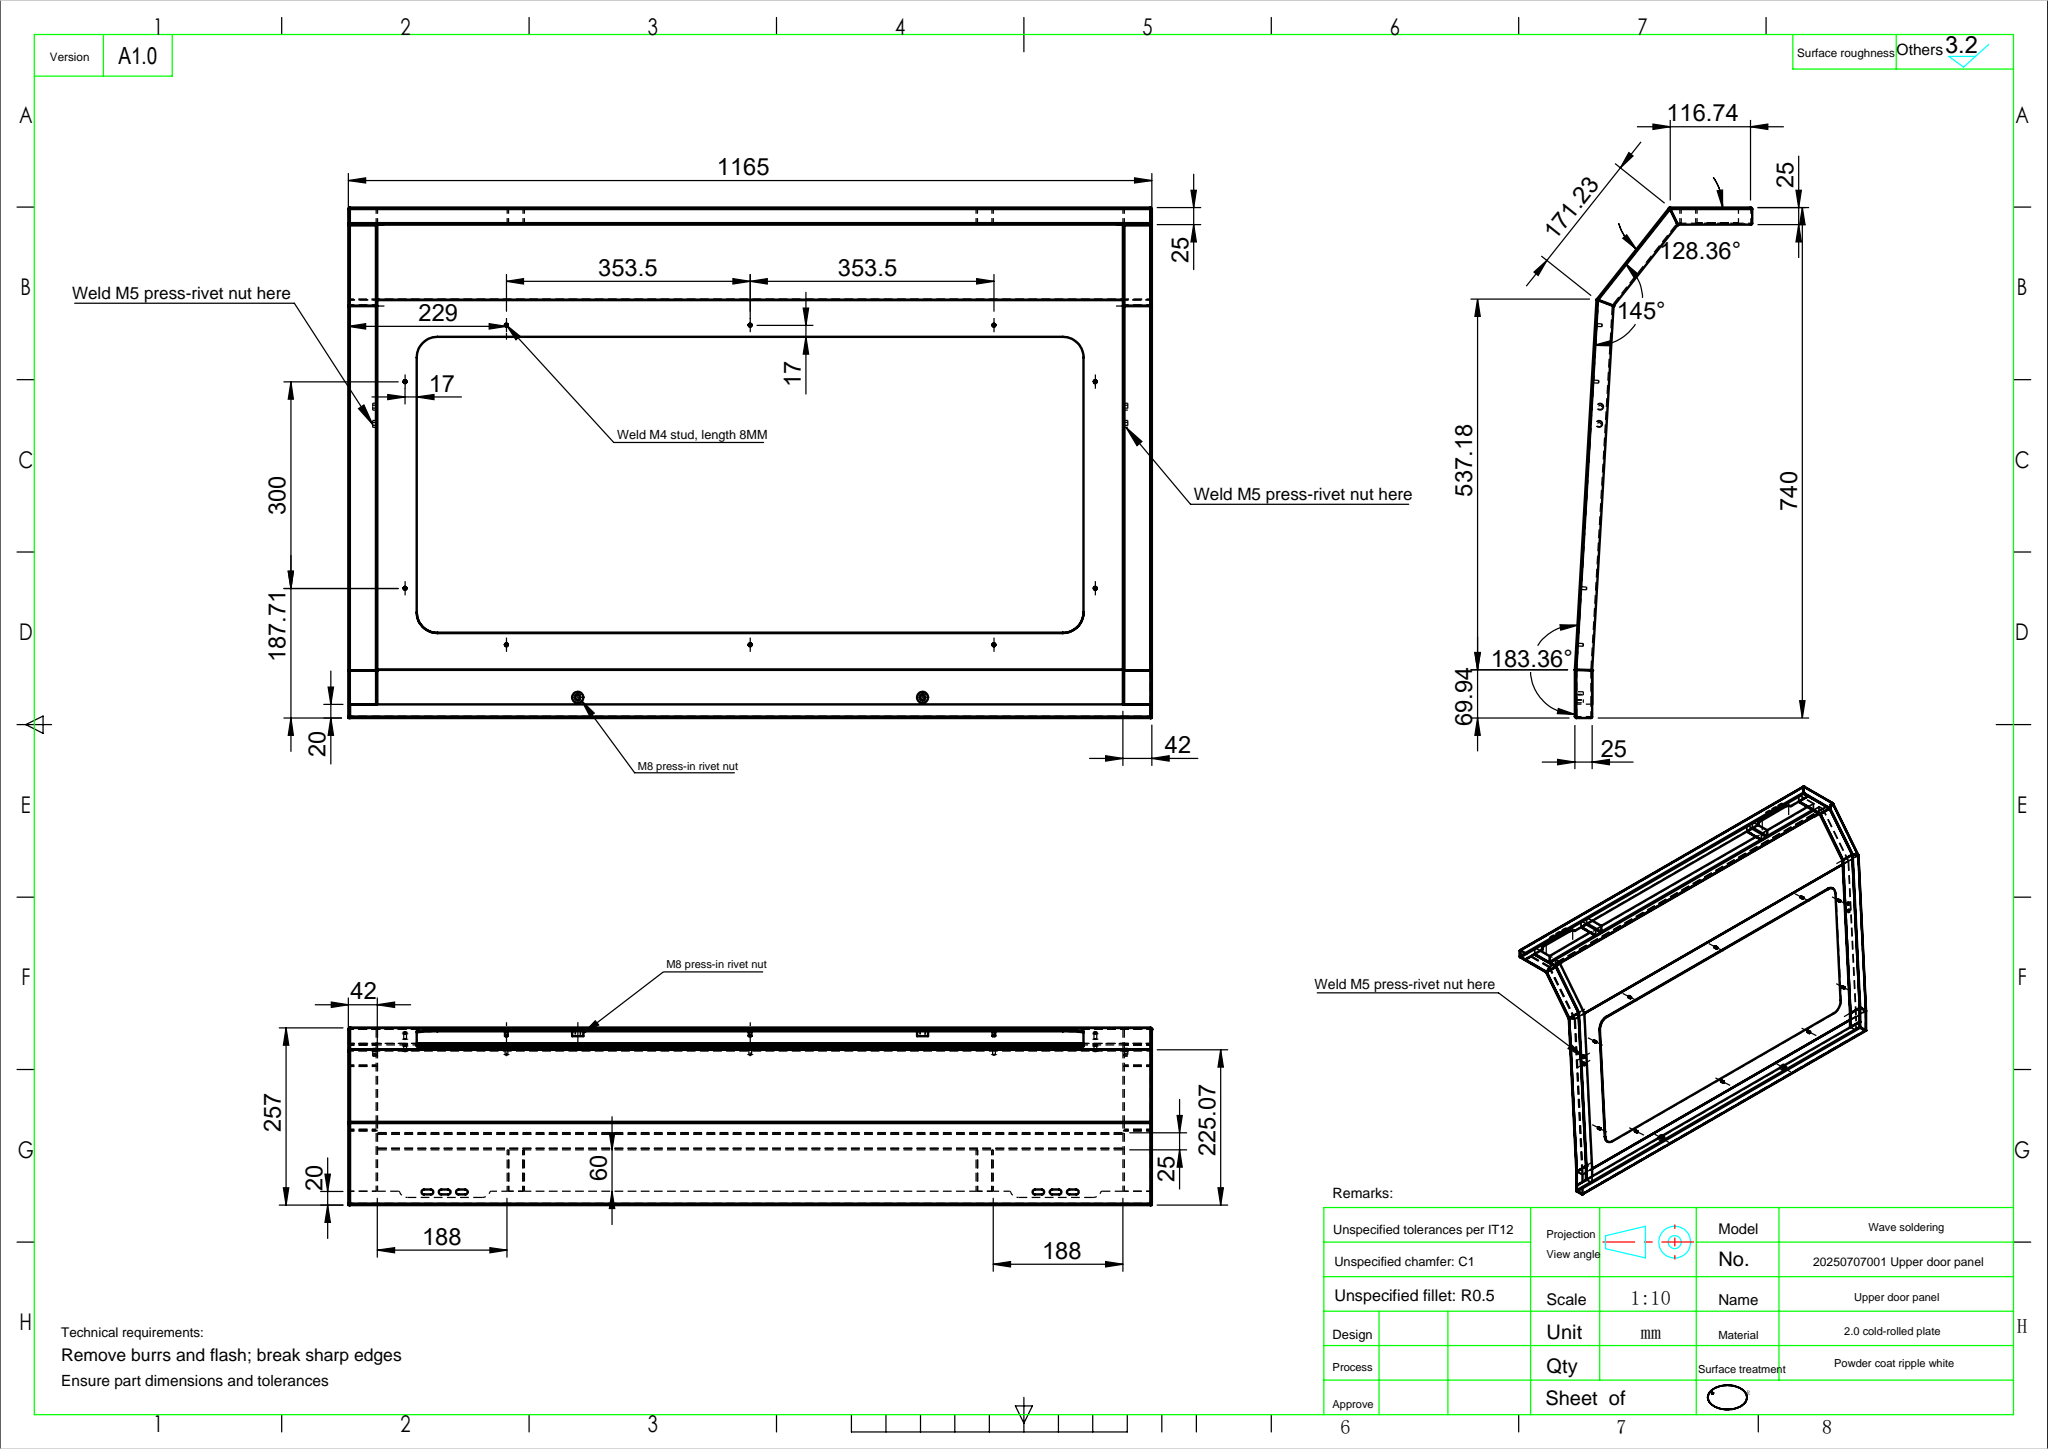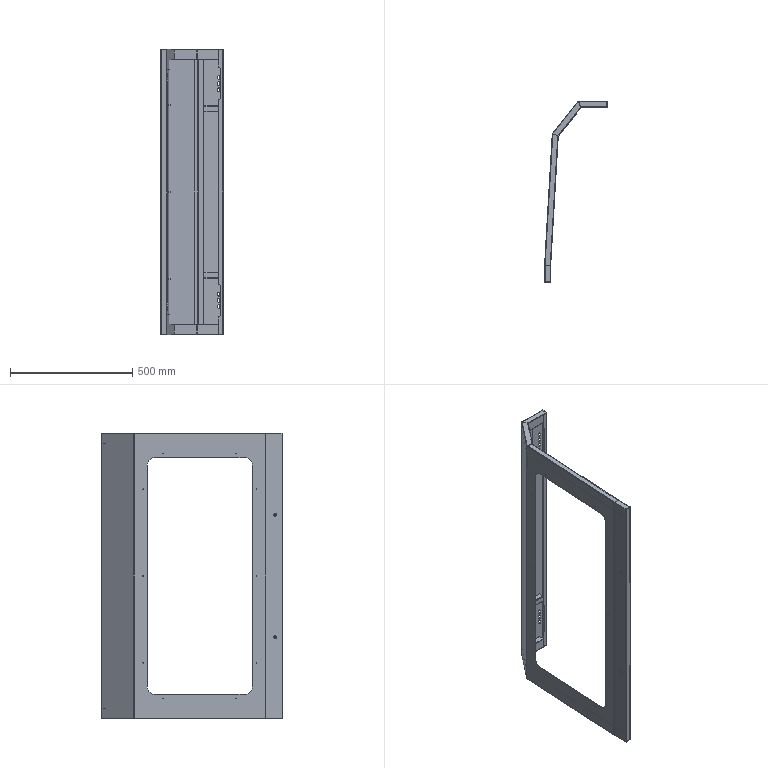Part | SolidWorks | features Chamfer 10, ICE 7, FlatPattern 6, HoleWzd 5, SMBaseFlange 5, SheetMetal 5, Fillet 3, MirrorSolid 2, CornerFeat 1, EdgeFlange 1 | 18 solids | 476 faces | box 257 x 740 x 1165 mm | volume 1879483 mm3 | plane 270 | cylinder 174 | cone 20 | spline 12 | commonest cylinder face diameters 4 x48 0.4 x25 4.4 x25 7 x12 2 x8 4.2 x8